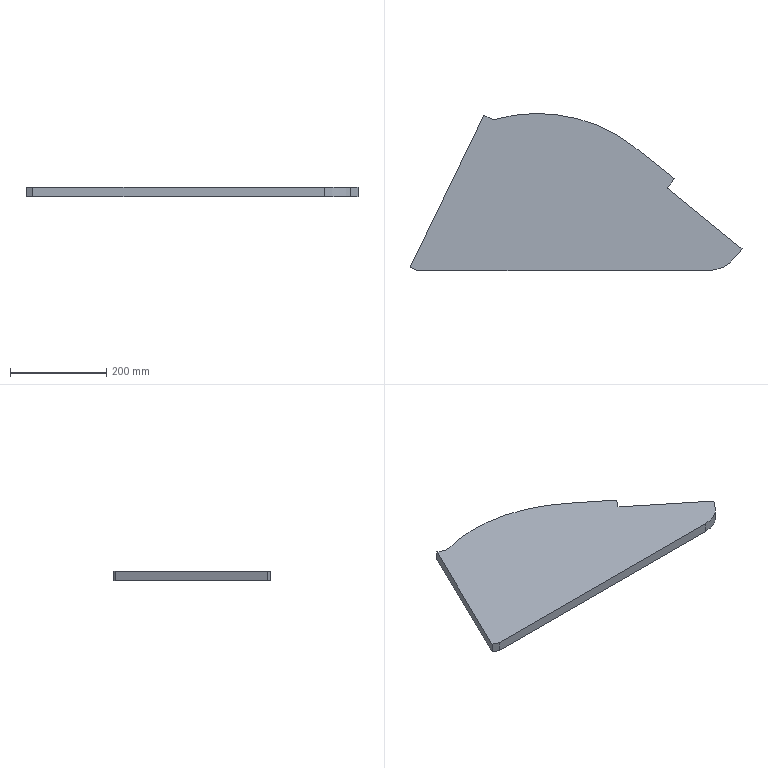Part | SolidWorks | features Extrusion 1 | 1 solid | 12 faces | box 689.12 x 326 x 20 mm | volume 3074154 mm3 | plane 10 | cylinder 2 | commonest cylinder face diameters 140 x1 652 x1
STEP:
#1=CARTESIAN_POINT('',(-14.12,6.856,0.));
#2=VERTEX_POINT('',#1);
#3=CARTESIAN_POINT('',(0.,0.,0.));
#4=VERTEX_POINT('',#3);
#5=CARTESIAN_POINT('',(0.,0.,0.));
#6=DIRECTION('',(0.8996,-0.4368,0.));
#7=VECTOR('',#6,1000.);
#8=LINE('',#5,#7);
#9=EDGE_CURVE('',#2,#4,#8,.T.);
#10=ORIENTED_EDGE('',*,*,#9,.T.);
#11=CARTESIAN_POINT('',(0.,0.,20.));
#12=VERTEX_POINT('',#11);
#13=CARTESIAN_POINT('',(0.,0.,20.));
#14=DIRECTION('',(0.,0.,-1.));
#15=VECTOR('',#14,1000.);
#16=LINE('',#13,#15);
#17=EDGE_CURVE('',#12,#4,#16,.T.);
#18=ORIENTED_EDGE('',*,*,#17,.F.);
#19=CARTESIAN_POINT('',(-14.12,6.856,20.));
#20=VERTEX_POINT('',#19);
#21=CARTESIAN_POINT('',(0.,0.,20.));
#22=DIRECTION('',(0.8996,-0.4368,0.));
#23=VECTOR('',#22,1000.);
#24=LINE('',#21,#23);
#25=EDGE_CURVE('',#20,#12,#24,.T.);
#26=ORIENTED_EDGE('',*,*,#25,.F.);
#27=CARTESIAN_POINT('',(-14.12,6.856,20.));
#28=DIRECTION('',(0.,0.,-1.));
#29=VECTOR('',#28,1000.);
#30=LINE('',#27,#29);
#31=EDGE_CURVE('',#20,#2,#30,.T.);
#32=ORIENTED_EDGE('',*,*,#31,.T.);
#33=EDGE_LOOP('',(#10,#18,#26,#32));
#34=FACE_OUTER_BOUND('',#33,.T.);
#35=CARTESIAN_POINT('',(0.,0.,20.));
#36=DIRECTION('',(0.4368,0.8996,0.));
#37=DIRECTION('',(-0.8996,0.4368,0.));
#38=AXIS2_PLACEMENT_3D('',#35,#36,#37);
#39=PLANE('',#38);
#40=ADVANCED_FACE('',(#34),#39,.F.);
#41=CARTESIAN_POINT('',(605.342,0.,0.));
#42=VERTEX_POINT('',#41);
#43=CARTESIAN_POINT('',(0.,0.,0.));
#44=DIRECTION('',(1.,0.,0.));
#45=VECTOR('',#44,1000.);
#46=LINE('',#43,#45);
#47=EDGE_CURVE('',#4,#42,#46,.T.);
#48=ORIENTED_EDGE('',*,*,#47,.T.);
#49=CARTESIAN_POINT('',(605.342,0.,20.));
#50=VERTEX_POINT('',#49);
#51=CARTESIAN_POINT('',(605.342,0.,20.));
#52=DIRECTION('',(0.,0.,-1.));
#53=VECTOR('',#52,1000.);
#54=LINE('',#51,#53);
#55=EDGE_CURVE('',#50,#42,#54,.T.);
#56=ORIENTED_EDGE('',*,*,#55,.F.);
#57=CARTESIAN_POINT('',(0.,0.,20.));
#58=DIRECTION('',(1.,0.,0.));
#59=VECTOR('',#58,1000.);
#60=LINE('',#57,#59);
#61=EDGE_CURVE('',#12,#50,#60,.T.);
#62=ORIENTED_EDGE('',*,*,#61,.F.);
#63=ORIENTED_EDGE('',*,*,#17,.T.);
#64=EDGE_LOOP('',(#48,#56,#62,#63));
#65=FACE_OUTER_BOUND('',#64,.T.);
#66=CARTESIAN_POINT('',(0.,0.,20.));
#67=DIRECTION('',(0.,1.,0.));
#68=DIRECTION('',(-1.,0.,0.));
#69=AXIS2_PLACEMENT_3D('',#66,#67,#68);
#70=PLANE('',#69);
#71=ADVANCED_FACE('',(#65),#70,.F.);
#72=CARTESIAN_POINT('',(660.209,26.531,0.));
#73=VERTEX_POINT('',#72);
#74=CARTESIAN_POINT('',(605.342,70.,0.));
#75=DIRECTION('',(0.,0.,1.));
#76=DIRECTION('',(1.,0.,0.));
#77=AXIS2_PLACEMENT_3D('',#74,#75,#76);
#78=CIRCLE('',#77,70.);
#79=EDGE_CURVE('',#42,#73,#78,.T.);
#80=ORIENTED_EDGE('',*,*,#79,.T.);
#81=CARTESIAN_POINT('',(660.209,26.531,20.));
#82=VERTEX_POINT('',#81);
#83=CARTESIAN_POINT('',(660.209,26.531,20.));
#84=DIRECTION('',(0.,0.,-1.));
#85=VECTOR('',#84,1000.);
#86=LINE('',#83,#85);
#87=EDGE_CURVE('',#82,#73,#86,.T.);
#88=ORIENTED_EDGE('',*,*,#87,.F.);
#89=CARTESIAN_POINT('',(605.342,70.,20.));
#90=DIRECTION('',(0.,0.,1.));
#91=DIRECTION('',(1.,0.,0.));
#92=AXIS2_PLACEMENT_3D('',#89,#90,#91);
#93=CIRCLE('',#92,70.);
#94=EDGE_CURVE('',#50,#82,#93,.T.);
#95=ORIENTED_EDGE('',*,*,#94,.F.);
#96=ORIENTED_EDGE('',*,*,#55,.T.);
#97=EDGE_LOOP('',(#80,#88,#95,#96));
#98=FACE_OUTER_BOUND('',#97,.T.);
#99=CARTESIAN_POINT('',(605.342,70.,20.));
#100=DIRECTION('',(0.,0.,-1.));
#101=DIRECTION('',(-1.,0.,0.));
#102=AXIS2_PLACEMENT_3D('',#99,#100,#101);
#103=CYLINDRICAL_SURFACE('',#102,70.);
#104=ADVANCED_FACE('',(#98),#103,.T.);
#105=CARTESIAN_POINT('',(675.,45.2,0.));
#106=VERTEX_POINT('',#105);
#107=CARTESIAN_POINT('',(675.,45.2,0.));
#108=DIRECTION('',(0.621,0.7838,0.));
#109=VECTOR('',#108,1000.);
#110=LINE('',#107,#109);
#111=EDGE_CURVE('',#73,#106,#110,.T.);
#112=ORIENTED_EDGE('',*,*,#111,.T.);
#113=CARTESIAN_POINT('',(675.,45.2,20.));
#114=VERTEX_POINT('',#113);
#115=CARTESIAN_POINT('',(675.,45.2,20.));
#116=DIRECTION('',(0.,0.,-1.));
#117=VECTOR('',#116,1000.);
#118=LINE('',#115,#117);
#119=EDGE_CURVE('',#114,#106,#118,.T.);
#120=ORIENTED_EDGE('',*,*,#119,.F.);
#121=CARTESIAN_POINT('',(675.,45.2,20.));
#122=DIRECTION('',(0.621,0.7838,0.));
#123=VECTOR('',#122,1000.);
#124=LINE('',#121,#123);
#125=EDGE_CURVE('',#82,#114,#124,.T.);
#126=ORIENTED_EDGE('',*,*,#125,.F.);
#127=ORIENTED_EDGE('',*,*,#87,.T.);
#128=EDGE_LOOP('',(#112,#120,#126,#127));
#129=FACE_OUTER_BOUND('',#128,.T.);
#130=CARTESIAN_POINT('',(675.,45.2,20.));
#131=DIRECTION('',(-0.7838,0.621,0.));
#132=DIRECTION('',(-0.621,-0.7838,0.));
#133=AXIS2_PLACEMENT_3D('',#130,#131,#132);
#134=PLANE('',#133);
#135=ADVANCED_FACE('',(#129),#134,.F.);
#136=CARTESIAN_POINT('',(519.4,170.9,0.));
#137=VERTEX_POINT('',#136);
#138=CARTESIAN_POINT('',(675.,45.2,0.));
#139=DIRECTION('',(-0.7779,0.6284,0.));
#140=VECTOR('',#139,1000.);
#141=LINE('',#138,#140);
#142=EDGE_CURVE('',#106,#137,#141,.T.);
#143=ORIENTED_EDGE('',*,*,#142,.T.);
#144=CARTESIAN_POINT('',(519.4,170.9,20.));
#145=VERTEX_POINT('',#144);
#146=CARTESIAN_POINT('',(519.4,170.9,20.));
#147=DIRECTION('',(0.,0.,-1.));
#148=VECTOR('',#147,1000.);
#149=LINE('',#146,#148);
#150=EDGE_CURVE('',#145,#137,#149,.T.);
#151=ORIENTED_EDGE('',*,*,#150,.F.);
#152=CARTESIAN_POINT('',(675.,45.2,20.));
#153=DIRECTION('',(-0.7779,0.6284,0.));
#154=VECTOR('',#153,1000.);
#155=LINE('',#152,#154);
#156=EDGE_CURVE('',#114,#145,#155,.T.);
#157=ORIENTED_EDGE('',*,*,#156,.F.);
#158=ORIENTED_EDGE('',*,*,#119,.T.);
#159=EDGE_LOOP('',(#143,#151,#157,#158));
#160=FACE_OUTER_BOUND('',#159,.T.);
#161=CARTESIAN_POINT('',(675.,45.2,20.));
#162=DIRECTION('',(-0.6284,-0.7779,0.));
#163=DIRECTION('',(0.7779,-0.6284,0.));
#164=AXIS2_PLACEMENT_3D('',#161,#162,#163);
#165=PLANE('',#164);
#166=ADVANCED_FACE('',(#160),#165,.F.);
#167=CARTESIAN_POINT('',(535.11,190.347,0.));
#168=VERTEX_POINT('',#167);
#169=CARTESIAN_POINT('',(519.4,170.9,0.));
#170=DIRECTION('',(0.6284,0.7779,0.));
#171=VECTOR('',#170,1000.);
#172=LINE('',#169,#171);
#173=EDGE_CURVE('',#137,#168,#172,.T.);
#174=ORIENTED_EDGE('',*,*,#173,.T.);
#175=CARTESIAN_POINT('',(535.11,190.347,20.));
#176=VERTEX_POINT('',#175);
#177=CARTESIAN_POINT('',(535.11,190.347,20.));
#178=DIRECTION('',(0.,0.,-1.));
#179=VECTOR('',#178,1000.);
#180=LINE('',#177,#179);
#181=EDGE_CURVE('',#176,#168,#180,.T.);
#182=ORIENTED_EDGE('',*,*,#181,.F.);
#183=CARTESIAN_POINT('',(519.4,170.9,20.));
#184=DIRECTION('',(0.6284,0.7779,0.));
#185=VECTOR('',#184,1000.);
#186=LINE('',#183,#185);
#187=EDGE_CURVE('',#145,#176,#186,.T.);
#188=ORIENTED_EDGE('',*,*,#187,.F.);
#189=ORIENTED_EDGE('',*,*,#150,.T.);
#190=EDGE_LOOP('',(#174,#182,#188,#189));
#191=FACE_OUTER_BOUND('',#190,.T.);
#192=CARTESIAN_POINT('',(519.4,170.9,20.));
#193=DIRECTION('',(-0.7779,0.6284,0.));
#194=DIRECTION('',(-0.6284,-0.7779,0.));
#195=AXIS2_PLACEMENT_3D('',#192,#193,#194);
#196=PLANE('',#195);
#197=ADVANCED_FACE('',(#191),#196,.F.);
#198=CARTESIAN_POINT('',(452.843,255.524,0.));
#199=VERTEX_POINT('',#198);
#200=CARTESIAN_POINT('',(535.11,190.347,0.));
#201=DIRECTION('',(-0.7838,0.621,0.));
#202=VECTOR('',#201,1000.);
#203=LINE('',#200,#202);
#204=EDGE_CURVE('',#168,#199,#203,.T.);
#205=ORIENTED_EDGE('',*,*,#204,.T.);
#206=CARTESIAN_POINT('',(452.843,255.524,20.));
#207=VERTEX_POINT('',#206);
#208=CARTESIAN_POINT('',(452.843,255.524,20.));
#209=DIRECTION('',(0.,0.,-1.));
#210=VECTOR('',#209,1000.);
#211=LINE('',#208,#210);
#212=EDGE_CURVE('',#207,#199,#211,.T.);
#213=ORIENTED_EDGE('',*,*,#212,.F.);
#214=CARTESIAN_POINT('',(535.11,190.347,20.));
#215=DIRECTION('',(-0.7838,0.621,0.));
#216=VECTOR('',#215,1000.);
#217=LINE('',#214,#216);
#218=EDGE_CURVE('',#176,#207,#217,.T.);
#219=ORIENTED_EDGE('',*,*,#218,.F.);
#220=ORIENTED_EDGE('',*,*,#181,.T.);
#221=EDGE_LOOP('',(#205,#213,#219,#220));
#222=FACE_OUTER_BOUND('',#221,.T.);
#223=CARTESIAN_POINT('',(535.11,190.347,20.));
#224=DIRECTION('',(-0.621,-0.7838,0.));
#225=DIRECTION('',(0.7838,-0.621,0.));
#226=AXIS2_PLACEMENT_3D('',#223,#224,#225);
#227=PLANE('',#226);
#228=ADVANCED_FACE('',(#222),#227,.F.);
#229=CARTESIAN_POINT('',(158.759,312.854,0.));
#230=VERTEX_POINT('',#229);
#231=CARTESIAN_POINT('',(250.4,0.,0.));
#232=DIRECTION('',(0.,0.,1.));
#233=DIRECTION('',(1.,0.,0.));
#234=AXIS2_PLACEMENT_3D('',#231,#232,#233);
#235=CIRCLE('',#234,326.);
#236=EDGE_CURVE('',#199,#230,#235,.T.);
#237=ORIENTED_EDGE('',*,*,#236,.T.);
#238=CARTESIAN_POINT('',(158.759,312.854,20.));
#239=VERTEX_POINT('',#238);
#240=CARTESIAN_POINT('',(158.759,312.854,20.));
#241=DIRECTION('',(0.,0.,-1.));
#242=VECTOR('',#241,1000.);
#243=LINE('',#240,#242);
#244=EDGE_CURVE('',#239,#230,#243,.T.);
#245=ORIENTED_EDGE('',*,*,#244,.F.);
#246=CARTESIAN_POINT('',(250.4,0.,20.));
#247=DIRECTION('',(0.,0.,1.));
#248=DIRECTION('',(1.,0.,0.));
#249=AXIS2_PLACEMENT_3D('',#246,#247,#248);
#250=CIRCLE('',#249,326.);
#251=EDGE_CURVE('',#207,#239,#250,.T.);
#252=ORIENTED_EDGE('',*,*,#251,.F.);
#253=ORIENTED_EDGE('',*,*,#212,.T.);
#254=EDGE_LOOP('',(#237,#245,#252,#253));
#255=FACE_OUTER_BOUND('',#254,.T.);
#256=CARTESIAN_POINT('',(250.4,0.,20.));
#257=DIRECTION('',(0.,0.,-1.));
#258=DIRECTION('',(-1.,0.,0.));
#259=AXIS2_PLACEMENT_3D('',#256,#257,#258);
#260=CYLINDRICAL_SURFACE('',#259,326.);
#261=ADVANCED_FACE('',(#255),#260,.T.);
#262=CARTESIAN_POINT('',(139.1,322.4,0.));
#263=VERTEX_POINT('',#262);
#264=CARTESIAN_POINT('',(139.1,322.4,0.));
#265=DIRECTION('',(-0.8996,0.4368,0.));
#266=VECTOR('',#265,1000.);
#267=LINE('',#264,#266);
#268=EDGE_CURVE('',#230,#263,#267,.T.);
#269=ORIENTED_EDGE('',*,*,#268,.T.);
#270=CARTESIAN_POINT('',(139.1,322.4,20.));
#271=VERTEX_POINT('',#270);
#272=CARTESIAN_POINT('',(139.1,322.4,20.));
#273=DIRECTION('',(0.,0.,-1.));
#274=VECTOR('',#273,1000.);
#275=LINE('',#272,#274);
#276=EDGE_CURVE('',#271,#263,#275,.T.);
#277=ORIENTED_EDGE('',*,*,#276,.F.);
#278=CARTESIAN_POINT('',(139.1,322.4,20.));
#279=DIRECTION('',(-0.8996,0.4368,0.));
#280=VECTOR('',#279,1000.);
#281=LINE('',#278,#280);
#282=EDGE_CURVE('',#239,#271,#281,.T.);
#283=ORIENTED_EDGE('',*,*,#282,.F.);
#284=ORIENTED_EDGE('',*,*,#244,.T.);
#285=EDGE_LOOP('',(#269,#277,#283,#284));
#286=FACE_OUTER_BOUND('',#285,.T.);
#287=CARTESIAN_POINT('',(139.1,322.4,20.));
#288=DIRECTION('',(-0.4368,-0.8996,0.));
#289=DIRECTION('',(0.8996,-0.4368,0.));
#290=AXIS2_PLACEMENT_3D('',#287,#288,#289);
#291=PLANE('',#290);
#292=ADVANCED_FACE('',(#286),#291,.F.);
#293=CARTESIAN_POINT('',(139.1,322.4,0.));
#294=DIRECTION('',(-0.4368,-0.8996,0.));
#295=VECTOR('',#294,1000.);
#296=LINE('',#293,#295);
#297=EDGE_CURVE('',#263,#2,#296,.T.);
#298=ORIENTED_EDGE('',*,*,#297,.T.);
#299=ORIENTED_EDGE('',*,*,#31,.F.);
#300=CARTESIAN_POINT('',(139.1,322.4,20.));
#301=DIRECTION('',(-0.4368,-0.8996,0.));
#302=VECTOR('',#301,1000.);
#303=LINE('',#300,#302);
#304=EDGE_CURVE('',#271,#20,#303,.T.);
#305=ORIENTED_EDGE('',*,*,#304,.F.);
#306=ORIENTED_EDGE('',*,*,#276,.T.);
#307=EDGE_LOOP('',(#298,#299,#305,#306));
#308=FACE_OUTER_BOUND('',#307,.T.);
#309=CARTESIAN_POINT('',(139.1,322.4,20.));
#310=DIRECTION('',(0.8996,-0.4368,0.));
#311=DIRECTION('',(0.4368,0.8996,0.));
#312=AXIS2_PLACEMENT_3D('',#309,#310,#311);
#313=PLANE('',#312);
#314=ADVANCED_FACE('',(#308),#313,.F.);
#315=ORIENTED_EDGE('',*,*,#25,.T.);
#316=ORIENTED_EDGE('',*,*,#61,.T.);
#317=ORIENTED_EDGE('',*,*,#94,.T.);
#318=ORIENTED_EDGE('',*,*,#125,.T.);
#319=ORIENTED_EDGE('',*,*,#156,.T.);
#320=ORIENTED_EDGE('',*,*,#187,.T.);
#321=ORIENTED_EDGE('',*,*,#218,.T.);
#322=ORIENTED_EDGE('',*,*,#251,.T.);
#323=ORIENTED_EDGE('',*,*,#282,.T.);
#324=ORIENTED_EDGE('',*,*,#304,.T.);
#325=EDGE_LOOP('',(#315,#316,#317,#318,#319,#320,#321,#322,#323,#324));
#326=FACE_OUTER_BOUND('',#325,.T.);
#327=CARTESIAN_POINT('',(250.4,0.,20.));
#328=DIRECTION('',(0.,0.,1.));
#329=DIRECTION('',(1.,0.,0.));
#330=AXIS2_PLACEMENT_3D('',#327,#328,#329);
#331=PLANE('',#330);
#332=ADVANCED_FACE('',(#326),#331,.T.);
#333=ORIENTED_EDGE('',*,*,#9,.F.);
#334=ORIENTED_EDGE('',*,*,#297,.F.);
#335=ORIENTED_EDGE('',*,*,#268,.F.);
#336=ORIENTED_EDGE('',*,*,#236,.F.);
#337=ORIENTED_EDGE('',*,*,#204,.F.);
#338=ORIENTED_EDGE('',*,*,#173,.F.);
#339=ORIENTED_EDGE('',*,*,#142,.F.);
#340=ORIENTED_EDGE('',*,*,#111,.F.);
#341=ORIENTED_EDGE('',*,*,#79,.F.);
#342=ORIENTED_EDGE('',*,*,#47,.F.);
#343=EDGE_LOOP('',(#333,#334,#335,#336,#337,#338,#339,#340,#341,#342));
#344=FACE_OUTER_BOUND('',#343,.T.);
#345=CARTESIAN_POINT('',(250.4,0.,0.));
#346=DIRECTION('',(0.,0.,1.));
#347=DIRECTION('',(1.,0.,0.));
#348=AXIS2_PLACEMENT_3D('',#345,#346,#347);
#349=PLANE('',#348);
#350=ADVANCED_FACE('',(#344),#349,.F.);
#351=CLOSED_SHELL('',(#40,#71,#104,#135,#166,#197,#228,#261,#292,#314,#332,#350));
#352=MANIFOLD_SOLID_BREP('',#351);
#353=CARTESIAN_POINT('',(0.,0.,0.));
#354=DIRECTION('',(0.,0.,1.));
#355=DIRECTION('',(1.,0.,0.));
#356=AXIS2_PLACEMENT_3D('',#353,#354,#355);
#357=(LENGTH_UNIT()NAMED_UNIT(*)SI_UNIT(.MILLI.,.METRE.));
#358=UNCERTAINTY_MEASURE_WITH_UNIT(LENGTH_MEASURE(0.00001),#357,'','');
#359=(NAMED_UNIT(*)PLANE_ANGLE_UNIT()SI_UNIT($,.RADIAN.));
#360=(NAMED_UNIT(*)SI_UNIT($,.STERADIAN.)SOLID_ANGLE_UNIT());
#361=(GEOMETRIC_REPRESENTATION_CONTEXT(3)GLOBAL_UNCERTAINTY_ASSIGNED_CONTEXT((#358))GLOBAL_UNIT_ASSIGNED_CONTEXT((#357,#359,#360))REPRESENTATION_CONTEXT('',''));
#362=ADVANCED_BREP_SHAPE_REPRESENTATION('',(#352,#356),#361);